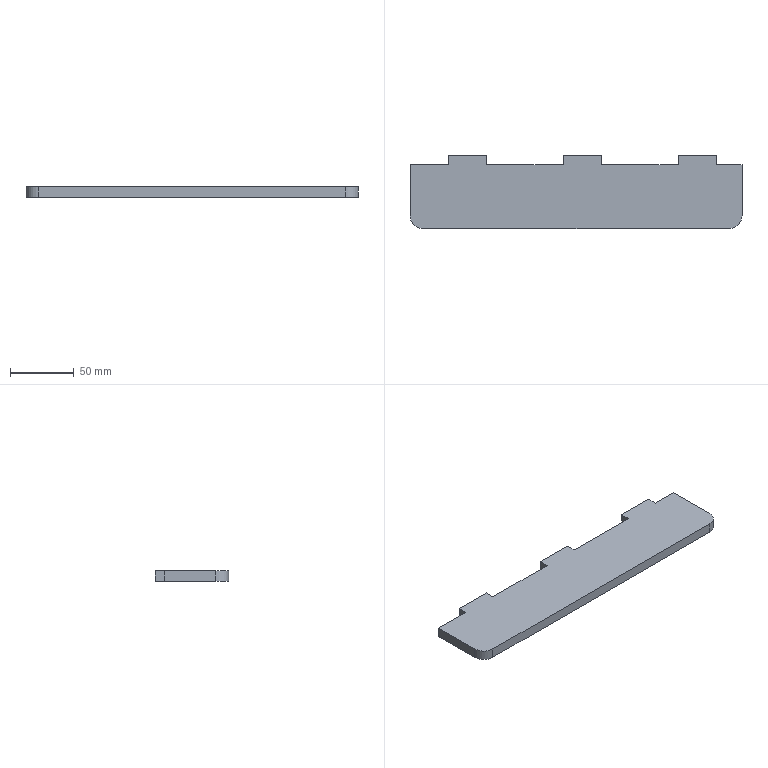Part | SolidWorks | features FlatPattern 1, SMBaseFlange 1, SheetMetal 1 | 1 solid | 20 faces | box 260 x 57.5 x 8 mm | volume 109057 mm3 | plane 18 | cylinder 2 | commonest cylinder face diameters 20 x2
STEP:
#1=CARTESIAN_POINT('',(192.817,-291.5,0.));
#2=VERTEX_POINT('',#1);
#3=CARTESIAN_POINT('',(172.817,-291.5,0.));
#4=VERTEX_POINT('',#3);
#5=CARTESIAN_POINT('',(172.817,-291.5,0.));
#6=DIRECTION('',(-1.,0.,0.));
#7=VECTOR('',#6,1000.);
#8=LINE('',#5,#7);
#9=EDGE_CURVE('',#2,#4,#8,.T.);
#10=ORIENTED_EDGE('',*,*,#9,.F.);
#11=CARTESIAN_POINT('',(192.817,-291.5,-8.));
#12=VERTEX_POINT('',#11);
#13=CARTESIAN_POINT('',(192.817,-291.5,-8.));
#14=DIRECTION('',(0.,0.,1.));
#15=VECTOR('',#14,1000.);
#16=LINE('',#13,#15);
#17=EDGE_CURVE('',#12,#2,#16,.T.);
#18=ORIENTED_EDGE('',*,*,#17,.F.);
#19=CARTESIAN_POINT('',(172.817,-291.5,-8.));
#20=VERTEX_POINT('',#19);
#21=CARTESIAN_POINT('',(172.817,-291.5,-8.));
#22=DIRECTION('',(-1.,0.,0.));
#23=VECTOR('',#22,1000.);
#24=LINE('',#21,#23);
#25=EDGE_CURVE('',#12,#20,#24,.T.);
#26=ORIENTED_EDGE('',*,*,#25,.T.);
#27=CARTESIAN_POINT('',(172.817,-291.5,-8.));
#28=DIRECTION('',(0.,0.,1.));
#29=VECTOR('',#28,1000.);
#30=LINE('',#27,#29);
#31=EDGE_CURVE('',#20,#4,#30,.T.);
#32=ORIENTED_EDGE('',*,*,#31,.T.);
#33=EDGE_LOOP('',(#10,#18,#26,#32));
#34=FACE_OUTER_BOUND('',#33,.T.);
#35=CARTESIAN_POINT('',(172.817,-291.5,-8.));
#36=DIRECTION('',(0.,1.,0.));
#37=DIRECTION('',(0.,0.,1.));
#38=AXIS2_PLACEMENT_3D('',#35,#36,#37);
#39=PLANE('',#38);
#40=ADVANCED_FACE('',(#34),#39,.T.);
#41=CARTESIAN_POINT('',(192.817,-331.5,0.));
#42=VERTEX_POINT('',#41);
#43=CARTESIAN_POINT('',(192.817,-291.5,0.));
#44=DIRECTION('',(0.,1.,0.));
#45=VECTOR('',#44,1000.);
#46=LINE('',#43,#45);
#47=EDGE_CURVE('',#42,#2,#46,.T.);
#48=ORIENTED_EDGE('',*,*,#47,.F.);
#49=CARTESIAN_POINT('',(192.817,-331.5,-8.));
#50=VERTEX_POINT('',#49);
#51=CARTESIAN_POINT('',(192.817,-331.5,-8.));
#52=DIRECTION('',(0.,0.,1.));
#53=VECTOR('',#52,1000.);
#54=LINE('',#51,#53);
#55=EDGE_CURVE('',#50,#42,#54,.T.);
#56=ORIENTED_EDGE('',*,*,#55,.F.);
#57=CARTESIAN_POINT('',(192.817,-291.5,-8.));
#58=DIRECTION('',(0.,1.,0.));
#59=VECTOR('',#58,1000.);
#60=LINE('',#57,#59);
#61=EDGE_CURVE('',#50,#12,#60,.T.);
#62=ORIENTED_EDGE('',*,*,#61,.T.);
#63=ORIENTED_EDGE('',*,*,#17,.T.);
#64=EDGE_LOOP('',(#48,#56,#62,#63));
#65=FACE_OUTER_BOUND('',#64,.T.);
#66=CARTESIAN_POINT('',(192.817,-291.5,-8.));
#67=DIRECTION('',(1.,0.,0.));
#68=DIRECTION('',(0.,1.,0.));
#69=AXIS2_PLACEMENT_3D('',#66,#67,#68);
#70=PLANE('',#69);
#71=ADVANCED_FACE('',(#65),#70,.T.);
#72=CARTESIAN_POINT('',(182.817,-341.5,0.));
#73=VERTEX_POINT('',#72);
#74=CARTESIAN_POINT('',(182.817,-331.5,0.));
#75=DIRECTION('',(0.,0.,1.));
#76=DIRECTION('',(-1.,0.,0.));
#77=AXIS2_PLACEMENT_3D('',#74,#75,#76);
#78=CIRCLE('',#77,10.);
#79=EDGE_CURVE('',#73,#42,#78,.T.);
#80=ORIENTED_EDGE('',*,*,#79,.F.);
#81=CARTESIAN_POINT('',(182.817,-341.5,-8.));
#82=VERTEX_POINT('',#81);
#83=CARTESIAN_POINT('',(182.817,-341.5,-8.));
#84=DIRECTION('',(0.,0.,1.));
#85=VECTOR('',#84,1000.);
#86=LINE('',#83,#85);
#87=EDGE_CURVE('',#82,#73,#86,.T.);
#88=ORIENTED_EDGE('',*,*,#87,.F.);
#89=CARTESIAN_POINT('',(182.817,-331.5,-8.));
#90=DIRECTION('',(0.,0.,1.));
#91=DIRECTION('',(-1.,0.,0.));
#92=AXIS2_PLACEMENT_3D('',#89,#90,#91);
#93=CIRCLE('',#92,10.);
#94=EDGE_CURVE('',#82,#50,#93,.T.);
#95=ORIENTED_EDGE('',*,*,#94,.T.);
#96=ORIENTED_EDGE('',*,*,#55,.T.);
#97=EDGE_LOOP('',(#80,#88,#95,#96));
#98=FACE_OUTER_BOUND('',#97,.T.);
#99=CARTESIAN_POINT('',(182.817,-331.5,-8.));
#100=DIRECTION('',(0.,0.,1.));
#101=DIRECTION('',(1.,0.,0.));
#102=AXIS2_PLACEMENT_3D('',#99,#100,#101);
#103=CYLINDRICAL_SURFACE('',#102,10.);
#104=ADVANCED_FACE('',(#98),#103,.T.);
#105=CARTESIAN_POINT('',(-57.183,-341.5,0.));
#106=VERTEX_POINT('',#105);
#107=CARTESIAN_POINT('',(182.817,-341.5,0.));
#108=DIRECTION('',(1.,0.,0.));
#109=VECTOR('',#108,1000.);
#110=LINE('',#107,#109);
#111=EDGE_CURVE('',#106,#73,#110,.T.);
#112=ORIENTED_EDGE('',*,*,#111,.F.);
#113=CARTESIAN_POINT('',(-57.183,-341.5,-8.));
#114=VERTEX_POINT('',#113);
#115=CARTESIAN_POINT('',(-57.183,-341.5,-8.));
#116=DIRECTION('',(0.,0.,1.));
#117=VECTOR('',#116,1000.);
#118=LINE('',#115,#117);
#119=EDGE_CURVE('',#114,#106,#118,.T.);
#120=ORIENTED_EDGE('',*,*,#119,.F.);
#121=CARTESIAN_POINT('',(182.817,-341.5,-8.));
#122=DIRECTION('',(1.,0.,0.));
#123=VECTOR('',#122,1000.);
#124=LINE('',#121,#123);
#125=EDGE_CURVE('',#114,#82,#124,.T.);
#126=ORIENTED_EDGE('',*,*,#125,.T.);
#127=ORIENTED_EDGE('',*,*,#87,.T.);
#128=EDGE_LOOP('',(#112,#120,#126,#127));
#129=FACE_OUTER_BOUND('',#128,.T.);
#130=CARTESIAN_POINT('',(182.817,-341.5,-8.));
#131=DIRECTION('',(0.,-1.,0.));
#132=DIRECTION('',(0.,0.,-1.));
#133=AXIS2_PLACEMENT_3D('',#130,#131,#132);
#134=PLANE('',#133);
#135=ADVANCED_FACE('',(#129),#134,.T.);
#136=CARTESIAN_POINT('',(-67.183,-331.5,0.));
#137=VERTEX_POINT('',#136);
#138=CARTESIAN_POINT('',(-57.183,-331.5,0.));
#139=DIRECTION('',(0.,0.,1.));
#140=DIRECTION('',(-1.,0.,0.));
#141=AXIS2_PLACEMENT_3D('',#138,#139,#140);
#142=CIRCLE('',#141,10.);
#143=EDGE_CURVE('',#137,#106,#142,.T.);
#144=ORIENTED_EDGE('',*,*,#143,.F.);
#145=CARTESIAN_POINT('',(-67.183,-331.5,-8.));
#146=VERTEX_POINT('',#145);
#147=CARTESIAN_POINT('',(-67.183,-331.5,-8.));
#148=DIRECTION('',(0.,0.,1.));
#149=VECTOR('',#148,1000.);
#150=LINE('',#147,#149);
#151=EDGE_CURVE('',#146,#137,#150,.T.);
#152=ORIENTED_EDGE('',*,*,#151,.F.);
#153=CARTESIAN_POINT('',(-57.183,-331.5,-8.));
#154=DIRECTION('',(0.,0.,1.));
#155=DIRECTION('',(-1.,0.,0.));
#156=AXIS2_PLACEMENT_3D('',#153,#154,#155);
#157=CIRCLE('',#156,10.);
#158=EDGE_CURVE('',#146,#114,#157,.T.);
#159=ORIENTED_EDGE('',*,*,#158,.T.);
#160=ORIENTED_EDGE('',*,*,#119,.T.);
#161=EDGE_LOOP('',(#144,#152,#159,#160));
#162=FACE_OUTER_BOUND('',#161,.T.);
#163=CARTESIAN_POINT('',(-57.183,-331.5,-8.));
#164=DIRECTION('',(0.,0.,1.));
#165=DIRECTION('',(1.,0.,0.));
#166=AXIS2_PLACEMENT_3D('',#163,#164,#165);
#167=CYLINDRICAL_SURFACE('',#166,10.);
#168=ADVANCED_FACE('',(#162),#167,.T.);
#169=CARTESIAN_POINT('',(-67.183,-291.5,0.));
#170=VERTEX_POINT('',#169);
#171=CARTESIAN_POINT('',(-67.183,-331.5,0.));
#172=DIRECTION('',(0.,-1.,0.));
#173=VECTOR('',#172,1000.);
#174=LINE('',#171,#173);
#175=EDGE_CURVE('',#170,#137,#174,.T.);
#176=ORIENTED_EDGE('',*,*,#175,.F.);
#177=CARTESIAN_POINT('',(-67.183,-291.5,-8.));
#178=VERTEX_POINT('',#177);
#179=CARTESIAN_POINT('',(-67.183,-291.5,-8.));
#180=DIRECTION('',(0.,0.,1.));
#181=VECTOR('',#180,1000.);
#182=LINE('',#179,#181);
#183=EDGE_CURVE('',#178,#170,#182,.T.);
#184=ORIENTED_EDGE('',*,*,#183,.F.);
#185=CARTESIAN_POINT('',(-67.183,-331.5,-8.));
#186=DIRECTION('',(0.,-1.,0.));
#187=VECTOR('',#186,1000.);
#188=LINE('',#185,#187);
#189=EDGE_CURVE('',#178,#146,#188,.T.);
#190=ORIENTED_EDGE('',*,*,#189,.T.);
#191=ORIENTED_EDGE('',*,*,#151,.T.);
#192=EDGE_LOOP('',(#176,#184,#190,#191));
#193=FACE_OUTER_BOUND('',#192,.T.);
#194=CARTESIAN_POINT('',(-67.183,-331.5,-8.));
#195=DIRECTION('',(-1.,0.,0.));
#196=DIRECTION('',(0.,0.,1.));
#197=AXIS2_PLACEMENT_3D('',#194,#195,#196);
#198=PLANE('',#197);
#199=ADVANCED_FACE('',(#193),#198,.T.);
#200=CARTESIAN_POINT('',(-37.183,-291.5,0.));
#201=VERTEX_POINT('',#200);
#202=CARTESIAN_POINT('',(-67.183,-291.5,0.));
#203=DIRECTION('',(-1.,0.,0.));
#204=VECTOR('',#203,1000.);
#205=LINE('',#202,#204);
#206=EDGE_CURVE('',#201,#170,#205,.T.);
#207=ORIENTED_EDGE('',*,*,#206,.F.);
#208=CARTESIAN_POINT('',(-37.183,-291.5,-8.));
#209=VERTEX_POINT('',#208);
#210=CARTESIAN_POINT('',(-37.183,-291.5,-8.));
#211=DIRECTION('',(0.,0.,1.));
#212=VECTOR('',#211,1000.);
#213=LINE('',#210,#212);
#214=EDGE_CURVE('',#209,#201,#213,.T.);
#215=ORIENTED_EDGE('',*,*,#214,.F.);
#216=CARTESIAN_POINT('',(-67.183,-291.5,-8.));
#217=DIRECTION('',(-1.,0.,0.));
#218=VECTOR('',#217,1000.);
#219=LINE('',#216,#218);
#220=EDGE_CURVE('',#209,#178,#219,.T.);
#221=ORIENTED_EDGE('',*,*,#220,.T.);
#222=ORIENTED_EDGE('',*,*,#183,.T.);
#223=EDGE_LOOP('',(#207,#215,#221,#222));
#224=FACE_OUTER_BOUND('',#223,.T.);
#225=CARTESIAN_POINT('',(-67.183,-291.5,-8.));
#226=DIRECTION('',(0.,1.,0.));
#227=DIRECTION('',(0.,0.,1.));
#228=AXIS2_PLACEMENT_3D('',#225,#226,#227);
#229=PLANE('',#228);
#230=ADVANCED_FACE('',(#224),#229,.T.);
#231=CARTESIAN_POINT('',(-37.183,-284.,0.));
#232=VERTEX_POINT('',#231);
#233=CARTESIAN_POINT('',(-37.183,-291.5,0.));
#234=DIRECTION('',(0.,-1.,0.));
#235=VECTOR('',#234,1000.);
#236=LINE('',#233,#235);
#237=EDGE_CURVE('',#232,#201,#236,.T.);
#238=ORIENTED_EDGE('',*,*,#237,.F.);
#239=CARTESIAN_POINT('',(-37.183,-284.,-8.));
#240=VERTEX_POINT('',#239);
#241=CARTESIAN_POINT('',(-37.183,-284.,-8.));
#242=DIRECTION('',(0.,0.,1.));
#243=VECTOR('',#242,1000.);
#244=LINE('',#241,#243);
#245=EDGE_CURVE('',#240,#232,#244,.T.);
#246=ORIENTED_EDGE('',*,*,#245,.F.);
#247=CARTESIAN_POINT('',(-37.183,-291.5,-8.));
#248=DIRECTION('',(0.,-1.,0.));
#249=VECTOR('',#248,1000.);
#250=LINE('',#247,#249);
#251=EDGE_CURVE('',#240,#209,#250,.T.);
#252=ORIENTED_EDGE('',*,*,#251,.T.);
#253=ORIENTED_EDGE('',*,*,#214,.T.);
#254=EDGE_LOOP('',(#238,#246,#252,#253));
#255=FACE_OUTER_BOUND('',#254,.T.);
#256=CARTESIAN_POINT('',(-37.183,-291.5,-8.));
#257=DIRECTION('',(-1.,0.,0.));
#258=DIRECTION('',(0.,0.,1.));
#259=AXIS2_PLACEMENT_3D('',#256,#257,#258);
#260=PLANE('',#259);
#261=ADVANCED_FACE('',(#255),#260,.T.);
#262=CARTESIAN_POINT('',(-7.183,-284.,0.));
#263=VERTEX_POINT('',#262);
#264=CARTESIAN_POINT('',(-37.183,-284.,0.));
#265=DIRECTION('',(-1.,0.,0.));
#266=VECTOR('',#265,1000.);
#267=LINE('',#264,#266);
#268=EDGE_CURVE('',#263,#232,#267,.T.);
#269=ORIENTED_EDGE('',*,*,#268,.F.);
#270=CARTESIAN_POINT('',(-7.183,-284.,-8.));
#271=VERTEX_POINT('',#270);
#272=CARTESIAN_POINT('',(-7.183,-284.,-8.));
#273=DIRECTION('',(0.,0.,1.));
#274=VECTOR('',#273,1000.);
#275=LINE('',#272,#274);
#276=EDGE_CURVE('',#271,#263,#275,.T.);
#277=ORIENTED_EDGE('',*,*,#276,.F.);
#278=CARTESIAN_POINT('',(-37.183,-284.,-8.));
#279=DIRECTION('',(-1.,0.,0.));
#280=VECTOR('',#279,1000.);
#281=LINE('',#278,#280);
#282=EDGE_CURVE('',#271,#240,#281,.T.);
#283=ORIENTED_EDGE('',*,*,#282,.T.);
#284=ORIENTED_EDGE('',*,*,#245,.T.);
#285=EDGE_LOOP('',(#269,#277,#283,#284));
#286=FACE_OUTER_BOUND('',#285,.T.);
#287=CARTESIAN_POINT('',(-37.183,-284.,-8.));
#288=DIRECTION('',(0.,1.,0.));
#289=DIRECTION('',(0.,0.,1.));
#290=AXIS2_PLACEMENT_3D('',#287,#288,#289);
#291=PLANE('',#290);
#292=ADVANCED_FACE('',(#286),#291,.T.);
#293=CARTESIAN_POINT('',(-7.183,-291.5,0.));
#294=VERTEX_POINT('',#293);
#295=CARTESIAN_POINT('',(-7.183,-284.,0.));
#296=DIRECTION('',(0.,1.,0.));
#297=VECTOR('',#296,1000.);
#298=LINE('',#295,#297);
#299=EDGE_CURVE('',#294,#263,#298,.T.);
#300=ORIENTED_EDGE('',*,*,#299,.F.);
#301=CARTESIAN_POINT('',(-7.183,-291.5,-8.));
#302=VERTEX_POINT('',#301);
#303=CARTESIAN_POINT('',(-7.183,-291.5,-8.));
#304=DIRECTION('',(0.,0.,1.));
#305=VECTOR('',#304,1000.);
#306=LINE('',#303,#305);
#307=EDGE_CURVE('',#302,#294,#306,.T.);
#308=ORIENTED_EDGE('',*,*,#307,.F.);
#309=CARTESIAN_POINT('',(-7.183,-284.,-8.));
#310=DIRECTION('',(0.,1.,0.));
#311=VECTOR('',#310,1000.);
#312=LINE('',#309,#311);
#313=EDGE_CURVE('',#302,#271,#312,.T.);
#314=ORIENTED_EDGE('',*,*,#313,.T.);
#315=ORIENTED_EDGE('',*,*,#276,.T.);
#316=EDGE_LOOP('',(#300,#308,#314,#315));
#317=FACE_OUTER_BOUND('',#316,.T.);
#318=CARTESIAN_POINT('',(-7.183,-284.,-8.));
#319=DIRECTION('',(1.,0.,0.));
#320=DIRECTION('',(0.,0.,-1.));
#321=AXIS2_PLACEMENT_3D('',#318,#319,#320);
#322=PLANE('',#321);
#323=ADVANCED_FACE('',(#317),#322,.T.);
#324=CARTESIAN_POINT('',(52.817,-291.5,0.));
#325=VERTEX_POINT('',#324);
#326=CARTESIAN_POINT('',(-7.183,-291.5,0.));
#327=DIRECTION('',(-1.,0.,0.));
#328=VECTOR('',#327,1000.);
#329=LINE('',#326,#328);
#330=EDGE_CURVE('',#325,#294,#329,.T.);
#331=ORIENTED_EDGE('',*,*,#330,.F.);
#332=CARTESIAN_POINT('',(52.817,-291.5,-8.));
#333=VERTEX_POINT('',#332);
#334=CARTESIAN_POINT('',(52.817,-291.5,-8.));
#335=DIRECTION('',(0.,0.,1.));
#336=VECTOR('',#335,1000.);
#337=LINE('',#334,#336);
#338=EDGE_CURVE('',#333,#325,#337,.T.);
#339=ORIENTED_EDGE('',*,*,#338,.F.);
#340=CARTESIAN_POINT('',(-7.183,-291.5,-8.));
#341=DIRECTION('',(-1.,0.,0.));
#342=VECTOR('',#341,1000.);
#343=LINE('',#340,#342);
#344=EDGE_CURVE('',#333,#302,#343,.T.);
#345=ORIENTED_EDGE('',*,*,#344,.T.);
#346=ORIENTED_EDGE('',*,*,#307,.T.);
#347=EDGE_LOOP('',(#331,#339,#345,#346));
#348=FACE_OUTER_BOUND('',#347,.T.);
#349=CARTESIAN_POINT('',(-7.183,-291.5,-8.));
#350=DIRECTION('',(0.,1.,0.));
#351=DIRECTION('',(0.,0.,1.));
#352=AXIS2_PLACEMENT_3D('',#349,#350,#351);
#353=PLANE('',#352);
#354=ADVANCED_FACE('',(#348),#353,.T.);
#355=CARTESIAN_POINT('',(52.817,-284.,0.));
#356=VERTEX_POINT('',#355);
#357=CARTESIAN_POINT('',(52.817,-291.5,0.));
#358=DIRECTION('',(0.,-1.,0.));
#359=VECTOR('',#358,1000.);
#360=LINE('',#357,#359);
#361=EDGE_CURVE('',#356,#325,#360,.T.);
#362=ORIENTED_EDGE('',*,*,#361,.F.);
#363=CARTESIAN_POINT('',(52.817,-284.,-8.));
#364=VERTEX_POINT('',#363);
#365=CARTESIAN_POINT('',(52.817,-284.,-8.));
#366=DIRECTION('',(0.,0.,1.));
#367=VECTOR('',#366,1000.);
#368=LINE('',#365,#367);
#369=EDGE_CURVE('',#364,#356,#368,.T.);
#370=ORIENTED_EDGE('',*,*,#369,.F.);
#371=CARTESIAN_POINT('',(52.817,-291.5,-8.));
#372=DIRECTION('',(0.,-1.,0.));
#373=VECTOR('',#372,1000.);
#374=LINE('',#371,#373);
#375=EDGE_CURVE('',#364,#333,#374,.T.);
#376=ORIENTED_EDGE('',*,*,#375,.T.);
#377=ORIENTED_EDGE('',*,*,#338,.T.);
#378=EDGE_LOOP('',(#362,#370,#376,#377));
#379=FACE_OUTER_BOUND('',#378,.T.);
#380=CARTESIAN_POINT('',(52.817,-291.5,-8.));
#381=DIRECTION('',(-1.,0.,0.));
#382=DIRECTION('',(0.,0.,1.));
#383=AXIS2_PLACEMENT_3D('',#380,#381,#382);
#384=PLANE('',#383);
#385=ADVANCED_FACE('',(#379),#384,.T.);
#386=CARTESIAN_POINT('',(82.817,-284.,0.));
#387=VERTEX_POINT('',#386);
#388=CARTESIAN_POINT('',(52.817,-284.,0.));
#389=DIRECTION('',(-1.,0.,0.));
#390=VECTOR('',#389,1000.);
#391=LINE('',#388,#390);
#392=EDGE_CURVE('',#387,#356,#391,.T.);
#393=ORIENTED_EDGE('',*,*,#392,.F.);
#394=CARTESIAN_POINT('',(82.817,-284.,-8.));
#395=VERTEX_POINT('',#394);
#396=CARTESIAN_POINT('',(82.817,-284.,-8.));
#397=DIRECTION('',(0.,0.,1.));
#398=VECTOR('',#397,1000.);
#399=LINE('',#396,#398);
#400=EDGE_CURVE('',#395,#387,#399,.T.);
#401=ORIENTED_EDGE('',*,*,#400,.F.);
#402=CARTESIAN_POINT('',(52.817,-284.,-8.));
#403=DIRECTION('',(-1.,0.,0.));
#404=VECTOR('',#403,1000.);
#405=LINE('',#402,#404);
#406=EDGE_CURVE('',#395,#364,#405,.T.);
#407=ORIENTED_EDGE('',*,*,#406,.T.);
#408=ORIENTED_EDGE('',*,*,#369,.T.);
#409=EDGE_LOOP('',(#393,#401,#407,#408));
#410=FACE_OUTER_BOUND('',#409,.T.);
#411=CARTESIAN_POINT('',(52.817,-284.,-8.));
#412=DIRECTION('',(0.,1.,0.));
#413=DIRECTION('',(0.,0.,1.));
#414=AXIS2_PLACEMENT_3D('',#411,#412,#413);
#415=PLANE('',#414);
#416=ADVANCED_FACE('',(#410),#415,.T.);
#417=CARTESIAN_POINT('',(82.817,-291.5,0.));
#418=VERTEX_POINT('',#417);
#419=CARTESIAN_POINT('',(82.817,-284.,0.));
#420=DIRECTION('',(0.,1.,0.));
#421=VECTOR('',#420,1000.);
#422=LINE('',#419,#421);
#423=EDGE_CURVE('',#418,#387,#422,.T.);
#424=ORIENTED_EDGE('',*,*,#423,.F.);
#425=CARTESIAN_POINT('',(82.817,-291.5,-8.));
#426=VERTEX_POINT('',#425);
#427=CARTESIAN_POINT('',(82.817,-291.5,-8.));
#428=DIRECTION('',(0.,0.,1.));
#429=VECTOR('',#428,1000.);
#430=LINE('',#427,#429);
#431=EDGE_CURVE('',#426,#418,#430,.T.);
#432=ORIENTED_EDGE('',*,*,#431,.F.);
#433=CARTESIAN_POINT('',(82.817,-284.,-8.));
#434=DIRECTION('',(0.,1.,0.));
#435=VECTOR('',#434,1000.);
#436=LINE('',#433,#435);
#437=EDGE_CURVE('',#426,#395,#436,.T.);
#438=ORIENTED_EDGE('',*,*,#437,.T.);
#439=ORIENTED_EDGE('',*,*,#400,.T.);
#440=EDGE_LOOP('',(#424,#432,#438,#439));
#441=FACE_OUTER_BOUND('',#440,.T.);
#442=CARTESIAN_POINT('',(82.817,-284.,-8.));
#443=DIRECTION('',(1.,0.,0.));
#444=DIRECTION('',(0.,1.,0.));
#445=AXIS2_PLACEMENT_3D('',#442,#443,#444);
#446=PLANE('',#445);
#447=ADVANCED_FACE('',(#441),#446,.T.);
#448=CARTESIAN_POINT('',(142.817,-291.5,0.));
#449=VERTEX_POINT('',#448);
#450=CARTESIAN_POINT('',(82.817,-291.5,0.));
#451=DIRECTION('',(-1.,0.,0.));
#452=VECTOR('',#451,1000.);
#453=LINE('',#450,#452);
#454=EDGE_CURVE('',#449,#418,#453,.T.);
#455=ORIENTED_EDGE('',*,*,#454,.F.);
#456=CARTESIAN_POINT('',(142.817,-291.5,-8.));
#457=VERTEX_POINT('',#456);
#458=CARTESIAN_POINT('',(142.817,-291.5,-8.));
#459=DIRECTION('',(0.,0.,1.));
#460=VECTOR('',#459,1000.);
#461=LINE('',#458,#460);
#462=EDGE_CURVE('',#457,#449,#461,.T.);
#463=ORIENTED_EDGE('',*,*,#462,.F.);
#464=CARTESIAN_POINT('',(82.817,-291.5,-8.));
#465=DIRECTION('',(-1.,0.,0.));
#466=VECTOR('',#465,1000.);
#467=LINE('',#464,#466);
#468=EDGE_CURVE('',#457,#426,#467,.T.);
#469=ORIENTED_EDGE('',*,*,#468,.T.);
#470=ORIENTED_EDGE('',*,*,#431,.T.);
#471=EDGE_LOOP('',(#455,#463,#469,#470));
#472=FACE_OUTER_BOUND('',#471,.T.);
#473=CARTESIAN_POINT('',(82.817,-291.5,-8.));
#474=DIRECTION('',(0.,1.,0.));
#475=DIRECTION('',(0.,0.,1.));
#476=AXIS2_PLACEMENT_3D('',#473,#474,#475);
#477=PLANE('',#476);
#478=ADVANCED_FACE('',(#472),#477,.T.);
#479=CARTESIAN_POINT('',(142.817,-284.,0.));
#480=VERTEX_POINT('',#479);
#481=CARTESIAN_POINT('',(142.817,-291.5,0.));
#482=DIRECTION('',(0.,-1.,0.));
#483=VECTOR('',#482,1000.);
#484=LINE('',#481,#483);
#485=EDGE_CURVE('',#480,#449,#484,.T.);
#486=ORIENTED_EDGE('',*,*,#485,.F.);
#487=CARTESIAN_POINT('',(142.817,-284.,-8.));
#488=VERTEX_POINT('',#487);
#489=CARTESIAN_POINT('',(142.817,-284.,-8.));
#490=DIRECTION('',(0.,0.,1.));
#491=VECTOR('',#490,1000.);
#492=LINE('',#489,#491);
#493=EDGE_CURVE('',#488,#480,#492,.T.);
#494=ORIENTED_EDGE('',*,*,#493,.F.);
#495=CARTESIAN_POINT('',(142.817,-291.5,-8.));
#496=DIRECTION('',(0.,-1.,0.));
#497=VECTOR('',#496,1000.);
#498=LINE('',#495,#497);
#499=EDGE_CURVE('',#488,#457,#498,.T.);
#500=ORIENTED_EDGE('',*,*,#499,.T.);
#501=ORIENTED_EDGE('',*,*,#462,.T.);
#502=EDGE_LOOP('',(#486,#494,#500,#501));
#503=FACE_OUTER_BOUND('',#502,.T.);
#504=CARTESIAN_POINT('',(142.817,-291.5,-8.));
#505=DIRECTION('',(-1.,0.,0.));
#506=DIRECTION('',(0.,0.,1.));
#507=AXIS2_PLACEMENT_3D('',#504,#505,#506);
#508=PLANE('',#507);
#509=ADVANCED_FACE('',(#503),#508,.T.);
#510=CARTESIAN_POINT('',(172.817,-284.,0.));
#511=VERTEX_POINT('',#510);
#512=CARTESIAN_POINT('',(142.817,-284.,0.));
#513=DIRECTION('',(-1.,0.,0.));
#514=VECTOR('',#513,1000.);
#515=LINE('',#512,#514);
#516=EDGE_CURVE('',#511,#480,#515,.T.);
#517=ORIENTED_EDGE('',*,*,#516,.F.);
#518=CARTESIAN_POINT('',(172.817,-284.,-8.));
#519=VERTEX_POINT('',#518);
#520=CARTESIAN_POINT('',(172.817,-284.,-8.));
#521=DIRECTION('',(0.,0.,1.));
#522=VECTOR('',#521,1000.);
#523=LINE('',#520,#522);
#524=EDGE_CURVE('',#519,#511,#523,.T.);
#525=ORIENTED_EDGE('',*,*,#524,.F.);
#526=CARTESIAN_POINT('',(142.817,-284.,-8.));
#527=DIRECTION('',(-1.,0.,0.));
#528=VECTOR('',#527,1000.);
#529=LINE('',#526,#528);
#530=EDGE_CURVE('',#519,#488,#529,.T.);
#531=ORIENTED_EDGE('',*,*,#530,.T.);
#532=ORIENTED_EDGE('',*,*,#493,.T.);
#533=EDGE_LOOP('',(#517,#525,#531,#532));
#534=FACE_OUTER_BOUND('',#533,.T.);
#535=CARTESIAN_POINT('',(142.817,-284.,-8.));
#536=DIRECTION('',(0.,1.,0.));
#537=DIRECTION('',(0.,0.,1.));
#538=AXIS2_PLACEMENT_3D('',#535,#536,#537);
#539=PLANE('',#538);
#540=ADVANCED_FACE('',(#534),#539,.T.);
#541=CARTESIAN_POINT('',(172.817,-284.,0.));
#542=DIRECTION('',(0.,1.,0.));
#543=VECTOR('',#542,1000.);
#544=LINE('',#541,#543);
#545=EDGE_CURVE('',#4,#511,#544,.T.);
#546=ORIENTED_EDGE('',*,*,#545,.F.);
#547=ORIENTED_EDGE('',*,*,#31,.F.);
#548=CARTESIAN_POINT('',(172.817,-284.,-8.));
#549=DIRECTION('',(0.,1.,0.));
#550=VECTOR('',#549,1000.);
#551=LINE('',#548,#550);
#552=EDGE_CURVE('',#20,#519,#551,.T.);
#553=ORIENTED_EDGE('',*,*,#552,.T.);
#554=ORIENTED_EDGE('',*,*,#524,.T.);
#555=EDGE_LOOP('',(#546,#547,#553,#554));
#556=FACE_OUTER_BOUND('',#555,.T.);
#557=CARTESIAN_POINT('',(172.817,-284.,-8.));
#558=DIRECTION('',(1.,0.,0.));
#559=DIRECTION('',(0.,0.,-1.));
#560=AXIS2_PLACEMENT_3D('',#557,#558,#559);
#561=PLANE('',#560);
#562=ADVANCED_FACE('',(#556),#561,.T.);
#563=ORIENTED_EDGE('',*,*,#25,.F.);
#564=ORIENTED_EDGE('',*,*,#61,.F.);
#565=ORIENTED_EDGE('',*,*,#94,.F.);
#566=ORIENTED_EDGE('',*,*,#125,.F.);
#567=ORIENTED_EDGE('',*,*,#158,.F.);
#568=ORIENTED_EDGE('',*,*,#189,.F.);
#569=ORIENTED_EDGE('',*,*,#220,.F.);
#570=ORIENTED_EDGE('',*,*,#251,.F.);
#571=ORIENTED_EDGE('',*,*,#282,.F.);
#572=ORIENTED_EDGE('',*,*,#313,.F.);
#573=ORIENTED_EDGE('',*,*,#344,.F.);
#574=ORIENTED_EDGE('',*,*,#375,.F.);
#575=ORIENTED_EDGE('',*,*,#406,.F.);
#576=ORIENTED_EDGE('',*,*,#437,.F.);
#577=ORIENTED_EDGE('',*,*,#468,.F.);
#578=ORIENTED_EDGE('',*,*,#499,.F.);
#579=ORIENTED_EDGE('',*,*,#530,.F.);
#580=ORIENTED_EDGE('',*,*,#552,.F.);
#581=EDGE_LOOP('',(#563,#564,#565,#566,#567,#568,#569,#570,#571,#572,#573,#574,#575,#576,#577,#578,#579,#580));
#582=FACE_OUTER_BOUND('',#581,.T.);
#583=CARTESIAN_POINT('',(182.817,-331.5,-8.));
#584=DIRECTION('',(0.,0.,-1.));
#585=DIRECTION('',(-1.,0.,0.));
#586=AXIS2_PLACEMENT_3D('',#583,#584,#585);
#587=PLANE('',#586);
#588=ADVANCED_FACE('',(#582),#587,.T.);
#589=ORIENTED_EDGE('',*,*,#9,.T.);
#590=ORIENTED_EDGE('',*,*,#545,.T.);
#591=ORIENTED_EDGE('',*,*,#516,.T.);
#592=ORIENTED_EDGE('',*,*,#485,.T.);
#593=ORIENTED_EDGE('',*,*,#454,.T.);
#594=ORIENTED_EDGE('',*,*,#423,.T.);
#595=ORIENTED_EDGE('',*,*,#392,.T.);
#596=ORIENTED_EDGE('',*,*,#361,.T.);
#597=ORIENTED_EDGE('',*,*,#330,.T.);
#598=ORIENTED_EDGE('',*,*,#299,.T.);
#599=ORIENTED_EDGE('',*,*,#268,.T.);
#600=ORIENTED_EDGE('',*,*,#237,.T.);
#601=ORIENTED_EDGE('',*,*,#206,.T.);
#602=ORIENTED_EDGE('',*,*,#175,.T.);
#603=ORIENTED_EDGE('',*,*,#143,.T.);
#604=ORIENTED_EDGE('',*,*,#111,.T.);
#605=ORIENTED_EDGE('',*,*,#79,.T.);
#606=ORIENTED_EDGE('',*,*,#47,.T.);
#607=EDGE_LOOP('',(#589,#590,#591,#592,#593,#594,#595,#596,#597,#598,#599,#600,#601,#602,#603,#604,#605,#606));
#608=FACE_OUTER_BOUND('',#607,.T.);
#609=CARTESIAN_POINT('',(182.817,-331.5,0.));
#610=DIRECTION('',(0.,0.,-1.));
#611=DIRECTION('',(-1.,0.,0.));
#612=AXIS2_PLACEMENT_3D('',#609,#610,#611);
#613=PLANE('',#612);
#614=ADVANCED_FACE('',(#608),#613,.F.);
#615=CLOSED_SHELL('',(#40,#71,#104,#135,#168,#199,#230,#261,#292,#323,#354,#385,#416,#447,#478,#509,#540,#562,#588,#614));
#616=MANIFOLD_SOLID_BREP('',#615);
#617=CARTESIAN_POINT('',(0.,0.,0.));
#618=DIRECTION('',(0.,0.,1.));
#619=DIRECTION('',(1.,0.,0.));
#620=AXIS2_PLACEMENT_3D('',#617,#618,#619);
#621=(LENGTH_UNIT()NAMED_UNIT(*)SI_UNIT(.MILLI.,.METRE.));
#622=UNCERTAINTY_MEASURE_WITH_UNIT(LENGTH_MEASURE(0.00001),#621,'','');
#623=(NAMED_UNIT(*)PLANE_ANGLE_UNIT()SI_UNIT($,.RADIAN.));
#624=(NAMED_UNIT(*)SI_UNIT($,.STERADIAN.)SOLID_ANGLE_UNIT());
#625=(GEOMETRIC_REPRESENTATION_CONTEXT(3)GLOBAL_UNCERTAINTY_ASSIGNED_CONTEXT((#622))GLOBAL_UNIT_ASSIGNED_CONTEXT((#621,#623,#624))REPRESENTATION_CONTEXT('',''));
#626=ADVANCED_BREP_SHAPE_REPRESENTATION('',(#616,#620),#625);